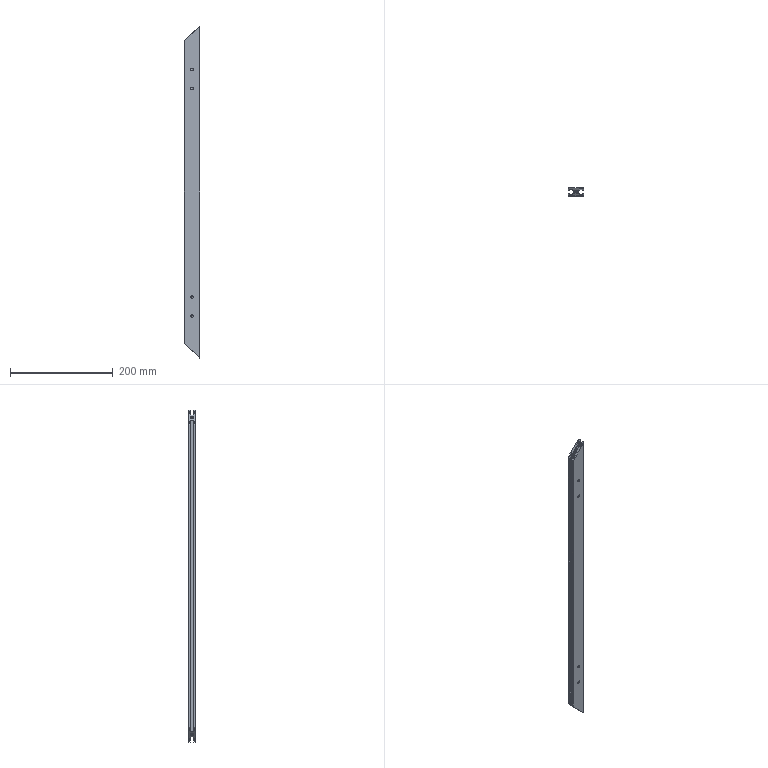Part | NX | features BREP 1 | 1 solid | 129 faces | box 30 x 15 x 647 mm | volume 148192 mm3 | cylinder 67 | plane 54 | cone 8 | commonest cylinder face diameters 5 x57 1 x6 2 x4